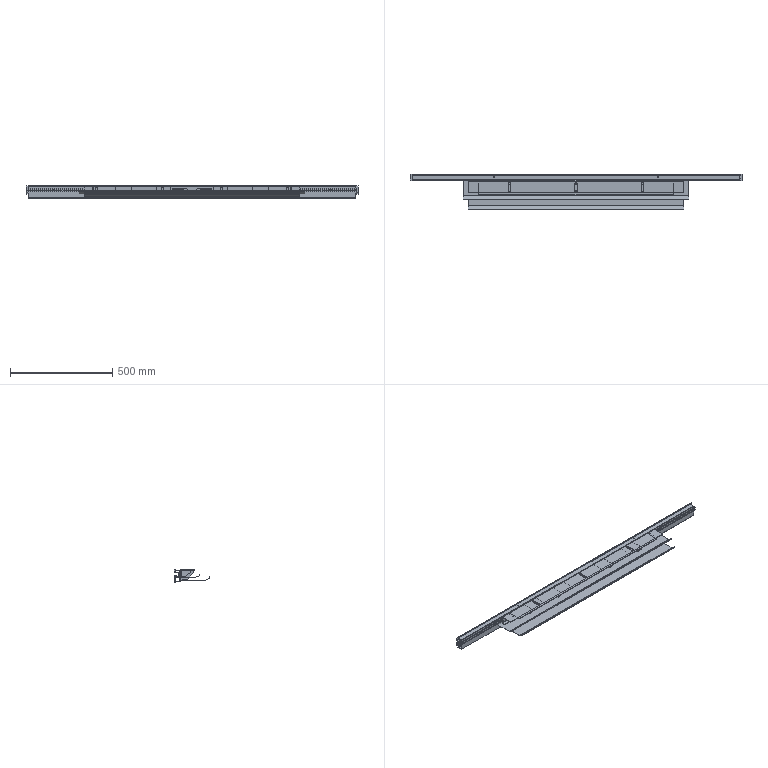Part | 17 solids | 530 faces | box 1620 x 170.821 x 60 mm | volume 1995290 mm3 | plane 324 | cylinder 206 | commonest cylinder face diameters 7 x43 6 x40 9 x30 10 x24 2 x22 11 x12